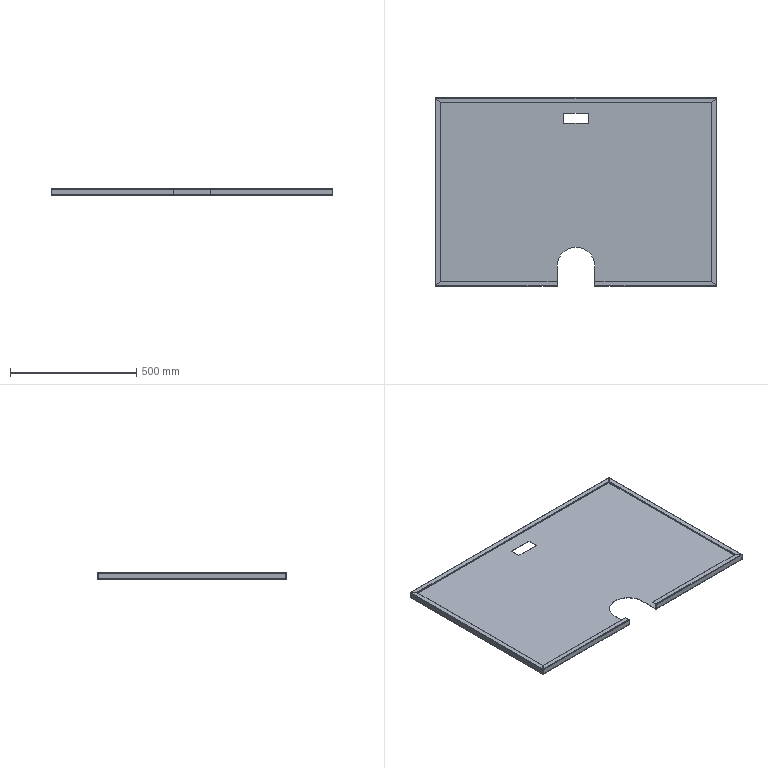Part | SolidWorks | features EdgeFlange 2, ICE 2, FlatPattern 1, SMBaseFlange 1, SheetMetal 1 | 1 solid | 94 faces | box 1116 x 747 x 25 mm | volume 1145204 mm3 | plane 57 | cylinder 21 | spline 16 | commonest cylinder face diameters 2 x10 4.4 x10 150 x1